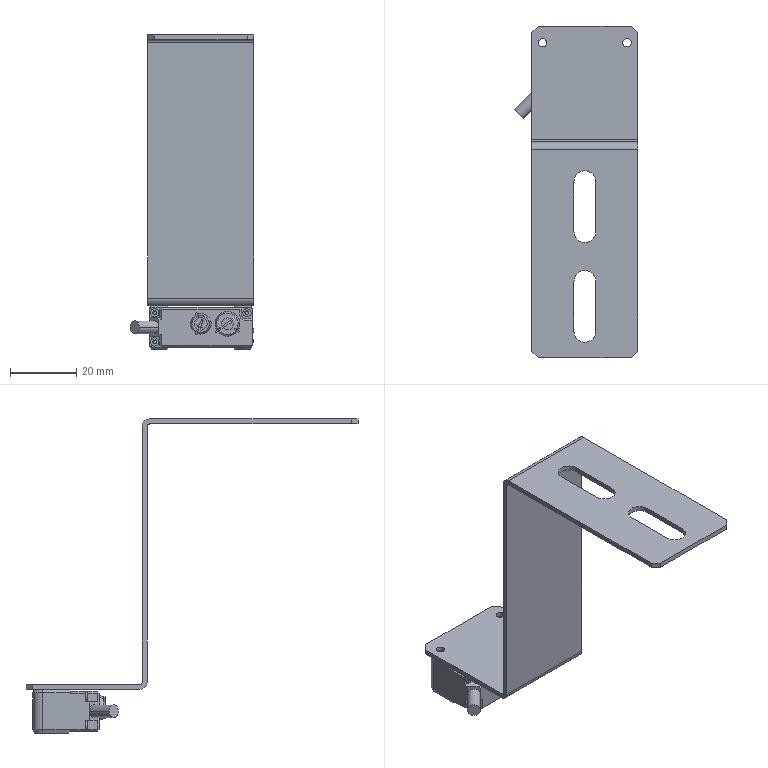Part | SolidWorks | 2 solids | 281 faces | box 37.32 x 100 x 94.6 mm | volume 15488 mm3 | plane 153 | cylinder 111 | cone 17 | commonest cylinder face diameters 0.3 x25 0.5 x22 2.5 x10 3.78 x7 6 x6 0.2 x5